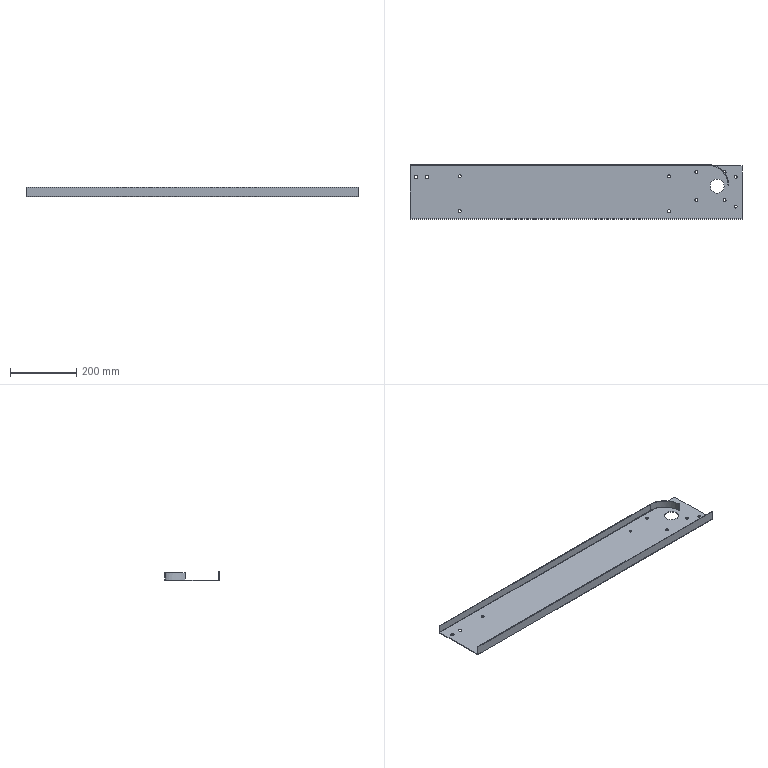Part | SolidWorks | features BaseBody 1 | 1 solid | 47 faces | box 1000 x 165 x 30 mm | volume 424200 mm3 | cylinder 32 | plane 14 | spline 1 | commonest cylinder face diameters 8.5 x12 9 x8 11 x4 1.473 x2 5.473 x2 42 x2